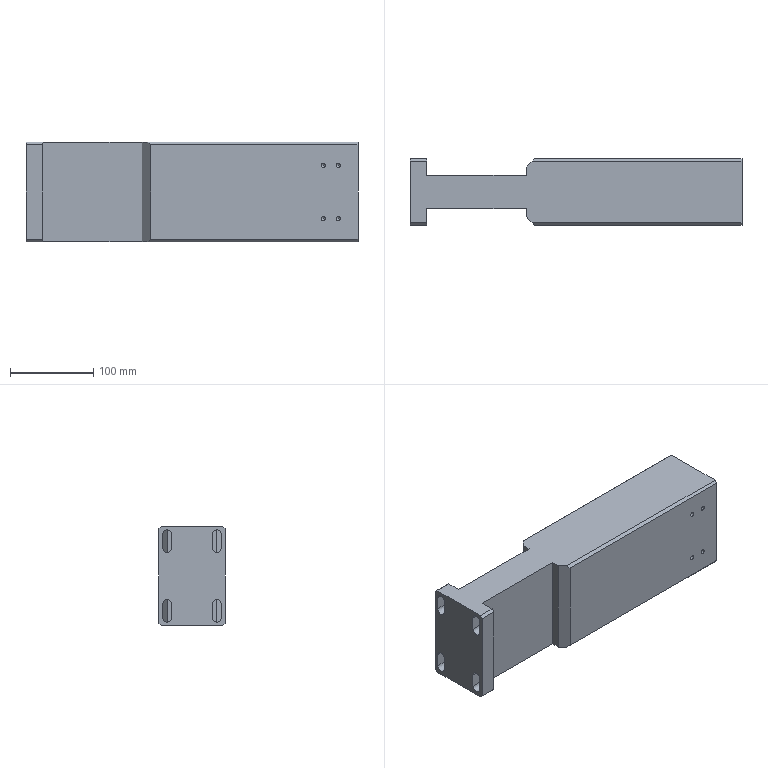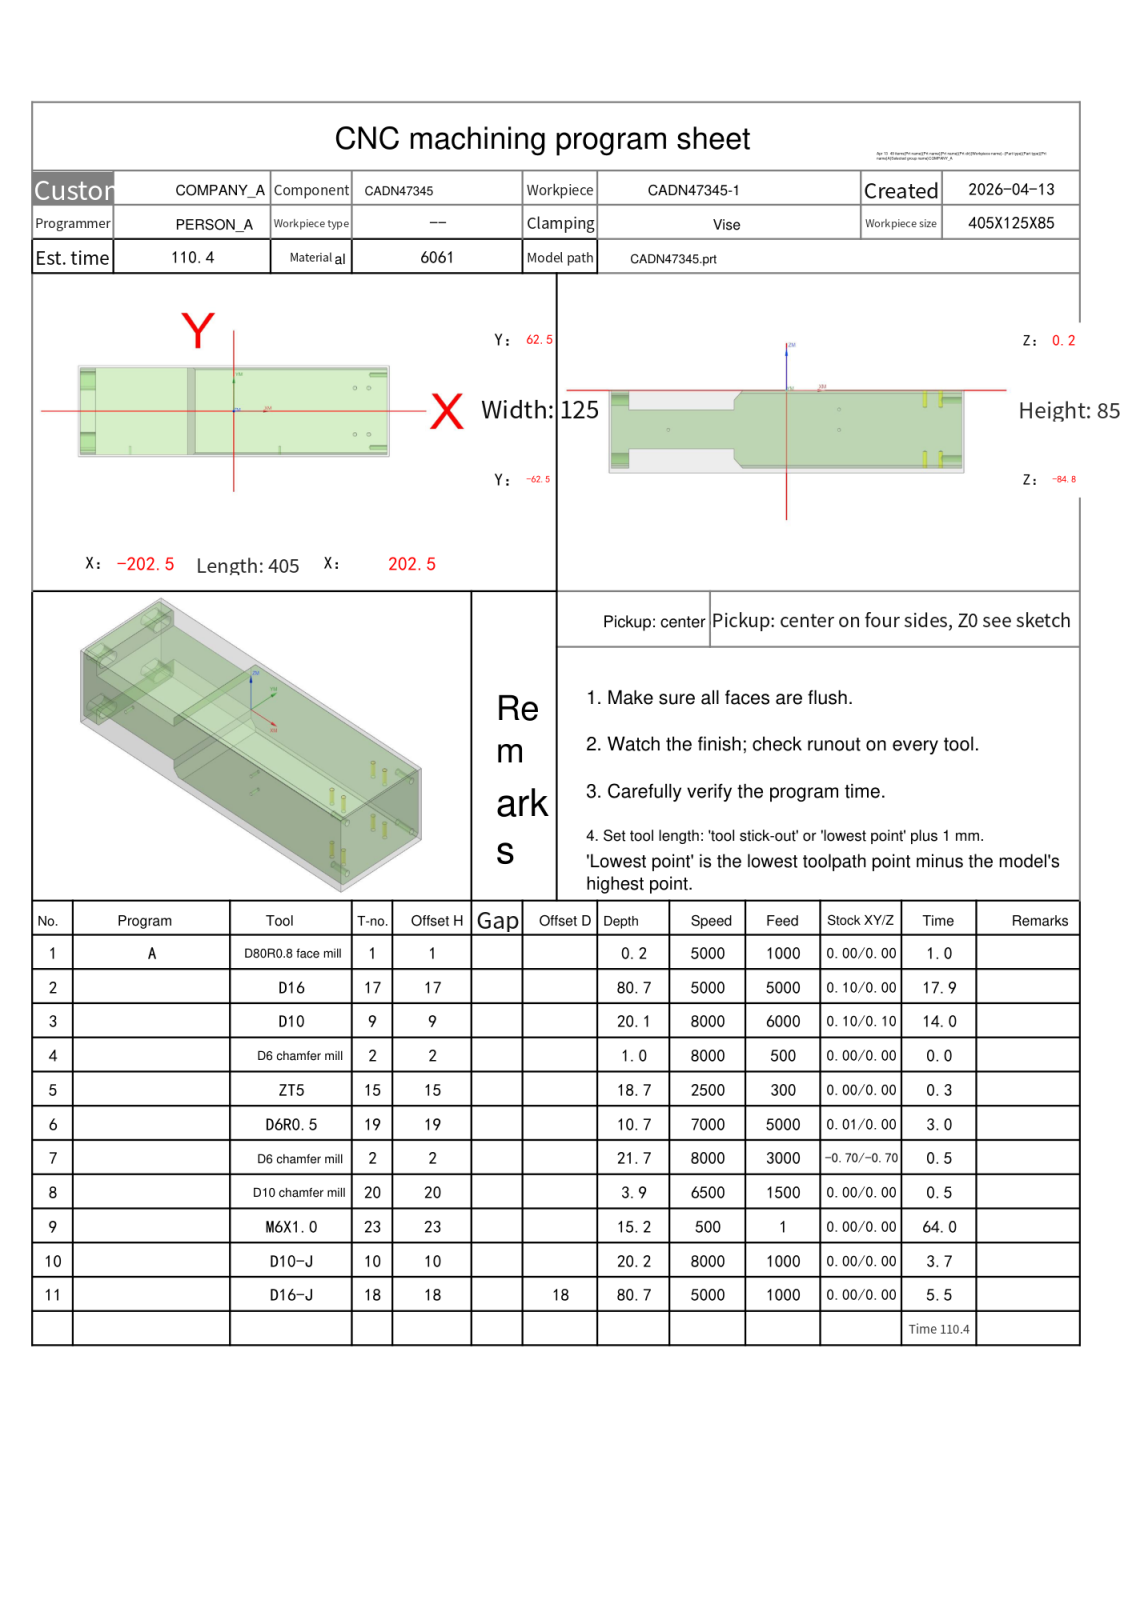NC program | NX | posted by the shop | part box 400 x 80 x 120 mm
Lines 711 to 1813 of 5986:
N3 T09 M06
(D10  D=10. R=0. H=09 ce=0.10 di=0.10)
G00 G90 G54 X-108.313 Y-74.5 M03 S8000
G43 H09 Z10.2
M08
Z.615
G01 Z-.585 F6000.
Y-67.08
G03 X-115.313 Y-60.08 I-7. J0.0
G01 X-174.823
G02 X-175.832 Y-63. I-5.247 J.18
G01 X-176.386
G02 X-180. Y-64.127 I-3.678 J5.437
G01 X-199.92
Y-63.
X-200.08
Y-62.727
X-199.921
X-199.92 Y-62.728
X-180. Y-62.727
G03 X-174.9 Y-57.585 I-.064 J5.164
G01 Y57.585
G03 X-180. Y62.727 I-5.164 J-.022
G01 X-199.92
X-199.921
X-199.999
X-200. Y62.728
X-200.001 Y62.727
X-200.08
Y63.
X-200.
Y64.127
Y63.
X-199.92
Y64.127
X-179.983
G02 X-176.386 Y63. I-.082 J-6.564
G01 X-175.849
G02 X-174.823 Y60.08 I-4.506 J-3.224
G01 X-174.002
X-166.904
X-65.09 Y60.082
X-64.793 Y60.08
X-58.152
G02 X-57.118 Y63. I5.554 J-.323
G01 X-54.305
G02 X-50.656 Y64.127 I3.649 J-5.344
G01 X200.011
X200.002 Y63.
X200.08
Y62.727
X200.001
X200. Y62.728
X-50.656 Y62.727
G03 X-55.727 Y57.656 I0.0 J-5.071
G01 Y-57.656
G03 X-50.656 Y-62.727 I5.071 J0.0
G01 X199.92
X199.921
X200.08
Y-63.
X199.92
Y-64.127
X-50.656
G02 X-54.305 Y-63. I0.0 J6.471
G01 X-57.118
G02 X-58.152 Y-60.08 I4.517 J3.243
G01 X-64.793
X-65.139 Y-60.082
X-65.389 Y-60.08
X-112.299
G02 X-113.112 Y-59.662 I.001 J1.
G01 X-117.515 Y-53.498
G03 X-118.327 Y-53.08 I-.813 J-.582
G01 X-166.904
G02 X-167.9 Y-52.084 I.004 J1.
G01 Y52.084
G02 X-166.904 Y53.08 I1. J-.004
G01 X-65.135 Y53.082
X-64.817 Y53.08
X-63.723
G02 X-62.727 Y52.084 I-.004 J-1.
G01 Y-52.084
G02 X-63.723 Y-53.08 I-1. J.004
G01 X-64.817
X-65.092 Y-53.082
X-65.366 Y-53.08
X-112.299
G02 X-113.112 Y-52.662 I.001 J1.
G01 X-117.515 Y-46.498
G03 X-118.327 Y-46.08 I-.813 J-.582
G01 X-159.905
G02 X-160.9 Y-45.085 I.005 J1.
G01 Y45.085
G02 X-159.905 Y46.08 I1. J-.005
G01 X-70.722 Y46.082
G02 X-69.727 Y45.087 I-.005 J-1.
G01 Y-45.085
G02 X-70.722 Y-46.08 I-1. J.005
G01 X-112.299
G02 X-113.112 Y-45.662 I.001 J1.
G01 X-117.515 Y-39.498
G03 X-118.327 Y-39.08 I-.813 J-.582
G01 X-152.905
G02 X-153.9 Y-38.085 I.005 J1.
G01 Y38.085
G02 X-152.905 Y39.08 I1. J-.005
G01 X-77.722 Y39.082
G02 X-76.727 Y38.087 I-.005 J-1.
G01 Y-38.085
G02 X-77.722 Y-39.08 I-1. J.005
G01 X-112.299
G02 X-113.112 Y-38.662 I0.0 J1.
G01 X-117.514 Y-32.498
G03 X-118.328 Y-32.08 I-.813 J-.582
G01 X-145.905
G02 X-146.9 Y-31.085 I.005 J1.
G01 Y31.086
G02 X-145.905 Y32.081 I1. J-.005
G01 X-84.722 Y32.082
G02 X-83.727 Y31.087 I-.005 J-1.
G01 Y-31.085
G02 X-84.722 Y-32.08 I-1. J.005
G01 X-112.299
G02 X-113.112 Y-31.662 I0.0 J1.
G01 X-117.514 Y-25.498
G03 X-118.328 Y-25.08 I-.814 J-.582
G01 X-138.905
G02 X-139.9 Y-24.085 I.005 J1.
G01 Y24.086
G02 X-138.905 Y25.081 I1. J-.005
G01 X-91.722 Y25.082
G02 X-90.727 Y24.087 I-.005 J-1.
G01 Y-24.085
G02 X-91.722 Y-25.08 I-1. J.005
G01 X-112.299
G02 X-113.112 Y-24.662 I0.0 J1.
G01 X-117.514 Y-18.498
G03 X-118.328 Y-18.08 I-.814 J-.582
G01 X-131.905
G02 X-132.9 Y-17.085 I.005 J1.
G01 Y17.086
G02 X-131.905 Y18.081 I1. J-.005
G01 X-98.721
G02 X-97.727 Y17.087 I-.005 J-1.
G01 Y-17.085
G02 X-98.721 Y-18.08 I-1. J.005
G01 X-112.299
G02 X-113.112 Y-17.662 I0.0 J1.
G01 X-117.514 Y-11.499
G03 X-118.328 Y-11.08 I-.814 J-.581
G01 X-124.905
G02 X-125.9 Y-10.085 I.005 J1.
G01 Y10.086
G02 X-124.905 Y11.081 I1. J-.005
G01 X-105.721
G02 X-104.727 Y10.087 I-.005 J-1.
G01 Y-10.085
G02 X-105.721 Y-11.08 I-1. J.005
G01 X-112.299
G02 X-113.112 Y-10.662 I0.0 J1.
G01 X-117.554 Y-4.443
G03 X-118.134 Y-4.052 I-.814 J-.582
G02 X-118.9 Y-3.085 I.234 J.972
G01 Y3.087
G02 X-117.905 Y4.081 I1. J-.005
G01 X-112.721
G02 X-111.727 Y3.087 I-.005 J-1.
G01 Y-3.085
G02 X-112.721 Y-4.08 I-1. J.005
G01 X-115.313
X-115.813
G03 X-122.813 Y-11.08 I0.0 J-7.
G01 Z.615
G00 Z3.
G01 X-108.313 Y-74.5
G00 Z.029
G01 Z-1.171
Y-67.08
G03 X-115.313 Y-60.08 I-7. J0.0
G01 X-174.823
G02 X-176.217 Y-63.466 I-5.247 J.18
X-180. Y-64.712 I-3.848 J5.318
G01 X-200.025
X-200. Y-63.312
X-180.
G03 X-174.9 Y-58.171 I-.064 J5.164
G01 Y58.171
G03 X-180. Y63.312 I-5.164 J-.022
G01 X-199.92
Y64.712
X-179.983
G02 X-176.234 Y63.479 I-.082 J-6.564
X-174.823 Y60.08 I-4.121 J-3.703
G01 X-166.905
X-65.09 Y60.082
X-64.793 Y60.08
X-58.152
G02 X-57.118 Y63. I5.554 J-.323
G01 X-55.626
G02 X-51.241 Y64.712 I4.385 J-4.759
G01 X199.92
Y63.312
X-51.241
G03 X-56.312 Y58.241 I0.0 J-5.071
G01 Y-58.241
G03 X-51.241 Y-63.312 I5.071 J0.0
G01 X200.
Y-64.712
X-51.241
G02 X-55.626 Y-63. I0.0 J6.471
G01 X-57.118
G02 X-58.152 Y-60.08 I4.517 J3.243
G01 X-64.793
X-65.139 Y-60.082
X-65.389 Y-60.08
X-112.299
G02 X-113.112 Y-59.662 I.001 J1.
G01 X-117.514 Y-53.499
G03 X-118.327 Y-53.081 I-.813 J-.582
G01 X-166.905 Y-53.08
G02 X-167.9 Y-52.085 I.005 J1.
G01 Y52.085
G02 X-166.905 Y53.08 I1. J-.005
G01 X-65.135 Y53.082
X-64.817 Y53.08
X-64.307
G02 X-63.312 Y52.084 I-.005 J-1.
G01 Y-52.084
G02 X-64.307 Y-53.08 I-1. J.005
G01 X-64.817
X-65.092 Y-53.082
X-112.299 Y-53.081
G02 X-113.112 Y-52.663 I.001 J1.
G01 X-117.514 Y-46.499
G03 X-118.327 Y-46.081 I-.813 J-.582
G01 X-159.905 Y-46.08
G02 X-160.9 Y-45.085 I.005 J1.
G01 Y45.085
G02 X-159.905 Y46.08 I1. J-.005
G01 X-71.307 Y46.082
G02 X-70.312 Y45.087 I-.005 J-1.
G01 Y-45.087
G02 X-71.307 Y-46.082 I-1. J.005
G01 X-112.299 Y-46.081
G02 X-113.112 Y-45.663 I.001 J1.
G01 X-117.514 Y-39.499
G03 X-118.327 Y-39.081 I-.813 J-.582
G01 X-152.905 Y-39.08
G02 X-153.9 Y-38.085 I.005 J1.
G01 Y38.086
G02 X-152.905 Y39.08 I1. J-.005
G01 X-78.307 Y39.082
G02 X-77.312 Y38.087 I-.005 J-1.
G01 Y-38.087
G02 X-78.307 Y-39.082 I-1. J.005
G01 X-112.299 Y-39.081
G02 X-113.112 Y-38.663 I.001 J1.
G01 X-117.514 Y-32.499
G03 X-118.327 Y-32.081 I-.813 J-.582
G01 X-145.905 Y-32.08
G02 X-146.9 Y-31.086 I.005 J1.
G01 Y31.086
G02 X-145.905 Y32.081 I1. J-.005
G01 X-85.307 Y32.082
G02 X-84.312 Y31.087 I-.005 J-1.
G01 Y-31.087
G02 X-85.307 Y-32.081 I-1. J.005
G01 X-112.299
G02 X-113.112 Y-31.663 I0.0 J1.
G01 X-117.514 Y-25.499
G03 X-118.327 Y-25.081 I-.814 J-.582
G01 X-138.906
G02 X-139.9 Y-24.086 I.006 J1.
G01 Y24.086
G02 X-138.906 Y25.081 I1. J-.005
G01 X-92.307 Y25.082
G02 X-91.312 Y24.087 I-.005 J-1.
G01 Y-24.087
G02 X-92.307 Y-25.081 I-1. J.005
G01 X-112.299
G02 X-113.112 Y-24.663 I0.0 J1.
G01 X-117.514 Y-18.499
G03 X-118.327 Y-18.081 I-.814 J-.582
G01 X-131.906
G02 X-132.9 Y-17.086 I.006 J1.
G01 Y17.086
G02 X-131.906 Y18.081 I1. J-.006
G01 X-99.306
G02 X-98.312 Y17.087 I-.006 J-1.
G01 Y-17.087
G02 X-99.306 Y-18.081 I-1. J.006
G01 X-112.298
G02 X-113.111 Y-17.663 I0.0 J1.
G01 X-117.514 Y-11.499
G03 X-118.327 Y-11.081 I-.814 J-.581
G01 X-124.906
G02 X-125.9 Y-10.086 I.006 J1.
G01 Y10.087
G02 X-124.906 Y11.081 I1. J-.006
G01 X-106.306
G02 X-105.312 Y10.087 I-.006 J-1.
G01 Y-10.087
G02 X-106.306 Y-11.081 I-1. J.006
G01 X-112.298
G02 X-113.111 Y-10.662 I0.0 J1.
G01 X-117.553 Y-4.444
G03 X-118.133 Y-4.053 I-.814 J-.581
G02 X-118.9 Y-3.087 I.233 J.972
G01 Y3.087
G02 X-117.906 Y4.081 I1. J-.006
G01 X-113.306
G02 X-112.312 Y3.087 I-.006 J-1.
G01 Y-3.087
G02 X-113.306 Y-4.081 I-1. J.006
G01 X-115.312
X-115.812
G03 X-122.812 Y-11.081 I0.0 J-7.
G01 Z.029
G00 Z3.
G01 X-108.313 Y-74.5
G00 Z-.556
G01 Z-1.756
Y-67.08
G03 X-115.313 Y-60.08 I-7. J0.0
G01 X-174.823
G02 X-180.07 Y-65.151 I-5.247 J.18
G01 X-180.08
X-200.
X-200.085 Y-65.156
X-200.08 Y-65.071
Y-63.897
X-199.92
X-180.
G03 X-174.9 Y-58.756 I-.064 J5.164
G01 Y58.756
G03 X-180. Y63.897 I-5.164 J-.022
G01 X-199.92
X-200.
X-200.08
Y65.071
X-200.085 Y65.156
X-200. Y65.151
X-180.079
G02 X-177.129 Y64.28 I-.06 J-5.639
X-174.823 Y60.08 I-3.226 J-4.504
G01 X-166.904
X-65.09 Y60.082
X-64.793 Y60.08
X-58.152
G02 X-55.897 Y64.236 I5.554 J-.324
X-52.574 Y65.157 I3.324 J-5.531
X-52.279 Y65.151 I0.0 J-6.453
G01 X200.
X200.085 Y65.156
X200.08 Y65.071
Y63.897
X199.92
X-51.827
G03 X-56.897 Y58.827 I0.0 J-5.071
G01 Y-58.827
G03 X-51.827 Y-63.897 I5.071 J0.0
G01 X200.
X200.08
Y-64.215
Y-65.071
X200.085 Y-65.156
X200. Y-65.151
X-52.283
X-53.186 Y-65.128
X-54.093 Y-64.999
X-54.999 Y-64.705
X-55.835 Y-64.281
G02 X-58.152 Y-60.08 I3.234 J4.523
G01 X-64.837
X-65.139 Y-60.082
X-65.389 Y-60.08
X-112.299
G02 X-113.112 Y-59.662 I.001 J1.
G01 X-117.515 Y-53.498
G03 X-118.327 Y-53.08 I-.813 J-.582
G01 X-166.904
G02 X-167.9 Y-52.084 I.004 J1.
G01 Y52.084
G02 X-166.904 Y53.08 I1. J-.004
G01 X-65.135 Y53.082
X-64.886 Y53.08
G02 X-63.897 Y52.084 I-.011 J-1.
G01 Y-52.084
G02 X-64.886 Y-53.08 I-1. J.004
G01 X-65.092 Y-53.082
X-65.366 Y-53.08
X-112.299
G02 X-113.112 Y-52.662 I.001 J1.
G01 X-117.515 Y-46.498
G03 X-118.327 Y-46.08 I-.813 J-.582
G01 X-159.905
G02 X-160.9 Y-45.085 I.005 J1.
G01 Y45.085
G02 X-159.905 Y46.08 I1. J-.005
G01 X-71.893 Y46.082
G02 X-70.897 Y45.087 I-.004 J-1.
G01 Y-45.085
G02 X-71.893 Y-46.08 I-1. J.005
G01 X-112.299
G02 X-113.112 Y-45.662 I0.0 J1.
G01 X-117.514 Y-39.498
G03 X-118.327 Y-39.08 I-.813 J-.582
G01 X-152.905
G02 X-153.9 Y-38.085 I.005 J1.
G01 Y38.085
G02 X-152.905 Y39.08 I1. J-.005
G01 X-78.893 Y39.082
G02 X-77.897 Y38.087 I-.005 J-1.
G01 Y-38.085
G02 X-78.893 Y-39.08 I-1. J.005
G01 X-112.299
G02 X-113.112 Y-38.662 I0.0 J1.
G01 X-117.514 Y-32.498
G03 X-118.328 Y-32.08 I-.813 J-.582
G01 X-145.905
G02 X-146.9 Y-31.085 I.005 J1.
G01 Y31.085
G02 X-145.905 Y32.081 I1. J-.005
G01 X-85.892 Y32.082
G02 X-84.897 Y31.087 I-.005 J-1.
G01 Y-31.085
G02 X-85.892 Y-32.08 I-1. J.005
G01 X-112.299
G02 X-113.112 Y-31.662 I0.0 J1.
G01 X-117.514 Y-25.498
G03 X-118.328 Y-25.08 I-.814 J-.582
G01 X-138.905
G02 X-139.9 Y-24.085 I.005 J1.
G01 Y24.086
G02 X-138.905 Y25.081 I1. J-.005
G01 X-92.892 Y25.082
G02 X-91.897 Y24.087 I-.005 J-1.
G01 Y-24.085
G02 X-92.892 Y-25.08 I-1. J.005
G01 X-112.299
G02 X-113.112 Y-24.662 I0.0 J1.
G01 X-117.514 Y-18.498
G03 X-118.328 Y-18.08 I-.814 J-.582
G01 X-131.905
G02 X-132.9 Y-17.085 I.005 J1.
G01 Y17.086
G02 X-131.905 Y18.081 I1. J-.005
G01 X-99.892
G02 X-98.897 Y17.087 I-.005 J-1.
G01 Y-17.085
G02 X-99.892 Y-18.08 I-1. J.005
G01 X-112.299
G02 X-113.112 Y-17.662 I0.0 J1.
G01 X-117.514 Y-11.499
G03 X-118.328 Y-11.08 I-.814 J-.582
G01 X-124.905
G02 X-125.9 Y-10.085 I.005 J1.
G01 Y10.086
G02 X-124.905 Y11.081 I1. J-.005
G01 X-106.892
G02 X-105.897 Y10.087 I-.005 J-1.
G01 Y-10.085
G02 X-106.892 Y-11.08 I-1. J.005
G01 X-112.299
G02 X-113.112 Y-10.661 I0.0 J1.
G01 X-117.554 Y-4.443
G03 X-118.134 Y-4.052 I-.814 J-.582
G02 X-118.9 Y-3.085 I.234 J.972
G01 Y3.086
G02 X-117.905 Y4.081 I1. J-.005
G01 X-113.892
G02 X-112.897 Y3.087 I-.005 J-1.
G01 Y-3.085
G02 X-113.892 Y-4.08 I-1. J.005
G01 X-115.313
X-115.813
G03 X-122.813 Y-11.08 I0.0 J-7.
G01 Z-.556
G00 Z3.
G01 X-108.313 Y-74.5
G00 Z-1.141
G01 Z-2.341
Y-67.08
G03 X-115.313 Y-60.08 I-7. J0.0
G01 X-174.823
G02 X-180.07 Y-65.151 I-5.247 J.18
G01 X-180.08
X-200.
X-200.085 Y-65.156
X-200.08 Y-65.071
Y-64.483
X-200.
X-199.92
X-180.
G03 X-174.9 Y-59.341 I-.069 J5.168
G01 Y59.341
G03 X-180. Y64.483 I-5.168 J-.027
G01 X-199.92
X-200.
X-200.08
Y65.071
X-200.085 Y65.156
X-200. Y65.151
X-180.079
G02 X-177.129 Y64.28 I-.06 J-5.639
X-174.823 Y60.08 I-3.226 J-4.504
G01 X-65.09 Y60.082
X-64.793 Y60.08
X-58.152
G02 X-55.897 Y64.236 I5.554 J-.324
X-52.574 Y65.157 I3.324 J-5.531
X-52.279 Y65.151 I0.0 J-6.453
G01 X200.
X200.085 Y65.156
X200.08 Y65.071
Y64.483
X200.
X-52.412
G03 X-57.483 Y59.412 I0.0 J-5.071
G01 Y-59.412
G03 X-52.412 Y-64.483 I5.071 J0.0
G01 X199.92
X200.
X200.08
Y-65.071
X200.085 Y-65.156
X200. Y-65.151
X-52.283
X-53.186 Y-65.128
X-54.093 Y-64.999
X-54.999 Y-64.705
X-55.835 Y-64.281
G02 X-58.152 Y-60.08 I3.234 J4.523
G01 X-64.793
X-65.092 Y-60.082
X-65.478 Y-60.08
X-112.299
G02 X-113.112 Y-59.662 I.001 J1.
G01 X-117.515 Y-53.498
G03 X-118.327 Y-53.08 I-.813 J-.582
G01 X-166.904
G02 X-167.9 Y-52.084 I.004 J1.
G01 Y52.085
G02 X-166.904 Y53.08 I1. J-.004
G01 X-65.478 Y53.082
G02 X-64.483 Y52.087 I-.004 J-1.
G01 Y-52.084
G02 X-65.478 Y-53.08 I-1. J.004
G01 X-112.299
G02 X-113.112 Y-52.662 I.001 J1.
G01 X-117.515 Y-46.498
G03 X-118.328 Y-46.08 I-.813 J-.582
G01 X-159.905
G02 X-160.9 Y-45.085 I.005 J1.
G01 Y45.085
G02 X-159.905 Y46.08 I1. J-.005
G01 X-72.478 Y46.082
G02 X-71.483 Y45.087 I-.005 J-1.
G01 Y-45.085
G02 X-72.478 Y-46.08 I-1. J.005
G01 X-112.299
G02 X-113.112 Y-45.662 I.001 J1.
G01 X-117.515 Y-39.498
G03 X-118.327 Y-39.08 I-.813 J-.582
G01 X-152.905
G02 X-153.9 Y-38.085 I.005 J1.
G01 Y38.086
G02 X-152.905 Y39.08 I1. J-.005
G01 X-79.477 Y39.082
G02 X-78.483 Y38.087 I-.005 J-1.
G01 Y-38.085
G02 X-79.477 Y-39.08 I-1. J.005
G01 X-112.299
G02 X-113.112 Y-38.662 I0.0 J1.
G01 X-117.515 Y-32.498
G03 X-118.328 Y-32.08 I-.813 J-.582
G01 X-145.905
G02 X-146.9 Y-31.085 I.005 J1.
G01 Y31.086
G02 X-145.905 Y32.081 I1. J-.005
G01 X-86.477 Y32.082
G02 X-85.483 Y31.087 I-.005 J-1.
G01 Y-31.085
G02 X-86.477 Y-32.08 I-1. J.005
G01 X-112.299
G02 X-113.112 Y-31.662 I0.0 J1.
G01 X-117.514 Y-25.498
G03 X-118.328 Y-25.08 I-.814 J-.582
G01 X-138.905
G02 X-139.9 Y-24.085 I.005 J1.
G01 Y24.086
G02 X-138.905 Y25.081 I1. J-.005
G01 X-93.477 Y25.082
G02 X-92.483 Y24.087 I-.005 J-1.
G01 Y-24.085
G02 X-93.477 Y-25.08 I-1. J.005
G01 X-112.299
G02 X-113.112 Y-24.662 I0.0 J1.
G01 X-117.514 Y-18.498
G03 X-118.328 Y-18.08 I-.814 J-.582
G01 X-131.906
G02 X-132.9 Y-17.086 I.006 J1.
G01 Y17.086
G02 X-131.906 Y18.081 I1. J-.006
G01 X-100.477
G02 X-99.483 Y17.087 I-.006 J-1.
G01 Y-17.086
G02 X-100.477 Y-18.08 I-1. J.006
G01 X-112.299
G02 X-113.112 Y-17.662 I0.0 J1.
G01 X-117.514 Y-11.499
G03 X-118.328 Y-11.08 I-.814 J-.582
G01 X-124.906
G02 X-125.9 Y-10.086 I.006 J1.
G01 Y10.087
G02 X-124.906 Y11.081 I1. J-.006
G01 X-107.477
G02 X-106.483 Y10.087 I-.006 J-1.
G01 Y-10.086
G02 X-107.477 Y-11.08 I-1. J.006
G01 X-112.299
G02 X-113.112 Y-10.661 I0.0 J1.
G01 X-117.554 Y-4.443
G03 X-118.134 Y-4.052 I-.814 J-.582
G02 X-118.9 Y-3.086 I.234 J.972
G01 Y3.087
G02 X-117.906 Y4.081 I1. J-.006
G01 X-114.477
G02 X-113.483 Y3.087 I-.006 J-1.
G01 Y-3.086
G02 X-114.477 Y-4.08 I-1. J.006
G01 X-115.313
X-115.813
G03 X-122.813 Y-11.08 I0.0 J-7.
G01 Z-1.141
G00 Z3.
G01 X-108.313 Y-74.5
G00 Z-1.726
G01 Z-2.926
Y-67.08
G03 X-115.313 Y-60.08 I-7. J0.0
G01 X-174.823
G02 X-175.832 Y-63. I-5.247 J.18
X-180.07 Y-65.151 I-4.238 J3.1
G01 X-180.08
X-200.
X-200.076 Y-65.163
X-200.078 Y-65.086
Y-65.067
X-180. Y-65.068
G03 X-174.9 Y-59.947 I-.021 J5.121
G01 Y-59.927
Y59.927
Y59.947
G03 X-180. Y65.068 I-5.121 J0.0
G01 X-200.078 Y65.067
X-200.079 Y65.086
X-200.076 Y65.163
X-200. Y65.151
X-180.079
G02 X-177.129 Y64.28 I-.06 J-5.639
X-175.849 Y63. I-3.226 J-4.504
X-174.823 Y60.08 I-4.506 J-3.224
G01 X-166.906
X-65.068 Y60.082
X-64.793 Y60.08
X-58.152
X-58.141 Y60.228
X-58.054 Y60.221
X-58.068 Y59.997
Y-59.997
X-58.053 Y-60.22
X-58.141 Y-60.226
X-58.152 Y-60.08
X-64.793
X-65.092 Y-60.082
X-65.389 Y-60.08
X-112.299
G02 X-113.112 Y-59.662 I.001 J1.
G01 X-117.515 Y-53.498
G03 X-118.327 Y-53.08 I-.813 J-.582
G01 X-166.905
G02 X-167.9 Y-52.085 I.005 J1.
G01 Y52.086
G02 X-166.905 Y53.08 I1. J-.005
G01 X-66.063 Y53.082
G02 X-65.068 Y52.087 I-.005 J-1.
G01 Y-52.085
G02 X-66.063 Y-53.08 I-1. J.005
G01 X-112.299
G02 X-113.112 Y-52.662 I.001 J1.
G01 X-117.515 Y-46.498
G03 X-118.327 Y-46.08 I-.813 J-.582
G01 X-159.906
G02 X-160.9 Y-45.086 I.006 J1.
G01 Y45.086
G02 X-159.906 Y46.08 I1. J-.006
G01 X-73.062 Y46.082
G02 X-72.068 Y45.088 I-.006 J-1.
G01 Y-45.086
G02 X-73.062 Y-46.08 I-1. J.006
G01 X-112.299
G02 X-113.112 Y-45.662 I.001 J1.
G01 X-117.515 Y-39.498
G03 X-118.327 Y-39.08 I-.813 J-.582
G01 X-152.906
G02 X-153.9 Y-38.086 I.006 J1.
G01 Y38.086
G02 X-152.906 Y39.08 I1. J-.006
G01 X-80.062 Y39.082
G02 X-79.068 Y38.088 I-.006 J-1.
G01 Y-38.086
G02 X-80.062 Y-39.08 I-1. J.006
G01 X-112.299
G02 X-113.112 Y-38.662 I0.0 J1.
G01 X-117.514 Y-32.498
G03 X-118.328 Y-32.08 I-.813 J-.582
G01 X-145.906
G02 X-146.9 Y-31.086 I.006 J1.
G01 Y31.086
G02 X-145.906 Y32.081 I1. J-.006
G01 X-87.062 Y32.082
G02 X-86.068 Y31.088 I-.006 J-1.
G01 Y-31.086
G02 X-87.062 Y-32.08 I-1. J.006
G01 X-112.299
G02 X-113.112 Y-31.662 I0.0 J1.
G01 X-117.514 Y-25.498
G03 X-118.328 Y-25.08 I-.814 J-.582
G01 X-138.906
G02 X-139.9 Y-24.086 I.006 J1.
G01 Y24.087
G02 X-138.906 Y25.081 I1. J-.006
G01 X-94.062 Y25.082
G02 X-93.068 Y24.088 I-.006 J-1.
G01 Y-24.086
G02 X-94.062 Y-25.08 I-1. J.006
G01 X-112.299
G02 X-113.112 Y-24.662 I0.0 J1.
G01 X-117.514 Y-18.498
G03 X-118.328 Y-18.08 I-.814 J-.582
G01 X-131.906
G02 X-132.9 Y-17.086 I.006 J1.
G01 Y17.087
G02 X-131.906 Y18.081 I1. J-.006
G01 X-101.062
G02 X-100.068 Y17.088 I-.006 J-1.
G01 Y-17.086
G02 X-101.062 Y-18.08 I-1. J.006
G01 X-112.299
G02 X-113.112 Y-17.662 I0.0 J1.
G01 X-117.514 Y-11.499
G03 X-118.328 Y-11.08 I-.814 J-.581
G01 X-124.906
G02 X-125.9 Y-10.086 I.006 J1.
G01 Y10.087
G02 X-124.906 Y11.081 I1. J-.006
G01 X-108.062
G02 X-107.068 Y10.087 I-.006 J-1.
G01 Y-10.086
G02 X-108.062 Y-11.08 I-1. J.006
G01 X-112.299
G02 X-113.112 Y-10.661 I0.0 J1.
G01 X-117.554 Y-4.443
G03 X-118.134 Y-4.052 I-.814 J-.582
G02 X-118.9 Y-3.086 I.234 J.972
G01 Y3.087
G02 X-117.906 Y4.081 I1. J-.006
G01 X-115.062
G02 X-114.068 Y3.087 I-.006 J-1.
G01 Y-3.086
G02 X-115.062 Y-4.08 I-1. J.006
G01 X-115.313
X-115.813
G03 X-122.813 Y-11.08 I0.0 J-7.
G01 Z-1.726
G00 Z3.
G01 X-108.313 Y-74.5
G00 Z-2.312
G01 Z-3.512
Y-67.08
G03 X-115.313 Y-60.08 I-7. J0.0
G01 X-174.823
X-174.9 Y-60.058
Y-59.927
Y60.068
X-174.823 Y60.08
X-65.09 Y60.082
X-64.793 Y60.08
X-58.653
Y59.92
Y-59.92
Y-60.08
X-64.793
X-65.092 Y-60.082
X-65.389 Y-60.08
X-112.299
G02 X-113.112 Y-59.662 I.001 J1.
G01 X-117.515 Y-53.498
G03 X-118.327 Y-53.08 I-.813 J-.582
G01 X-166.905
G02 X-167.9 Y-52.085 I.005 J1.
G01 Y52.085
G02 X-166.905 Y53.08 I1. J-.005
G01 X-66.648 Y53.082
G02 X-65.653 Y52.087 I-.005 J-1.
G01 Y-52.085
G02 X-66.648 Y-53.08 I-1. J.005
G01 X-112.299
G02 X-113.112 Y-52.662 I.001 J1.
G01 X-117.515 Y-46.498
G03 X-118.327 Y-46.08 I-.813 J-.582
G01 X-159.905
G02 X-160.9 Y-45.085 I.005 J1.
G01 Y45.086
G02 X-159.905 Y46.08 I1. J-.005
G01 X-73.648 Y46.082
G02 X-72.653 Y45.087 I-.005 J-1.
G01 Y-45.085
G02 X-73.648 Y-46.08 I-1. J.005
G01 X-112.299
G02 X-113.112 Y-45.662 I.001 J1.
G01 X-117.515 Y-39.498
G03 X-118.327 Y-39.08 I-.813 J-.582
G01 X-152.906
G02 X-153.9 Y-38.086 I.006 J1.
G01 Y38.086
G02 X-152.906 Y39.08 I1. J-.006
G01 X-80.648 Y39.082
G02 X-79.653 Y38.087 I-.006 J-1.
G01 Y-38.086
G02 X-80.648 Y-39.08 I-1. J.006
G01 X-112.299
G02 X-113.112 Y-38.662 I0.0 J1.
G01 X-117.514 Y-32.498
G03 X-118.328 Y-32.08 I-.813 J-.582
G01 X-145.906
G02 X-146.9 Y-31.086 I.006 J1.
G01 Y31.086
G02 X-145.906 Y32.081 I1. J-.006
G01 X-87.647 Y32.082
G02 X-86.653 Y31.087 I-.006 J-1.
G01 Y-31.086
G02 X-87.647 Y-32.08 I-1. J.006
G01 X-112.299
G02 X-113.112 Y-31.662 I0.0 J1.
G01 X-117.514 Y-25.498
G03 X-118.328 Y-25.08 I-.814 J-.582
G01 X-138.906
G02 X-139.9 Y-24.086 I.006 J1.
G01 Y24.087
G02 X-138.906 Y25.081 I1. J-.006
G01 X-94.647 Y25.082
G02 X-93.653 Y24.087 I-.006 J-1.
G01 Y-24.086
G02 X-94.647 Y-25.08 I-1. J.006
G01 X-112.299
G02 X-113.112 Y-24.662 I0.0 J1.
G01 X-117.514 Y-18.498
G03 X-118.328 Y-18.08 I-.814 J-.582
G01 X-131.906
G02 X-132.9 Y-17.086 I.006 J1.
G01 Y17.087
G02 X-131.906 Y18.081 I1. J-.006
G01 X-101.647
G02 X-100.653 Y17.087 I-.006 J-1.
G01 Y-17.086
G02 X-101.647 Y-18.08 I-1. J.006
G01 X-112.299
G02 X-113.112 Y-17.662 I0.0 J1.
G01 X-117.514 Y-11.499
G03 X-118.328 Y-11.08 I-.814 J-.582
G01 X-124.906
G02 X-125.9 Y-10.086 I.006 J1.
G01 Y10.087
G02 X-124.906 Y11.081 I1. J-.006
G01 X-108.647
G02 X-107.653 Y10.087 I-.006 J-1.
G01 Y-10.086
G02 X-108.647 Y-11.08 I-1. J.006
G01 X-112.315
G02 X-113.113 Y-10.682 I0.0 J1.
G01 X-117.927 Y-4.299
G03 X-118.312 Y-3.991 I-.798 J-.602
G02 X-118.9 Y-3.086 I.412 J.911
G01 Y3.087
G02 X-117.906 Y4.081 I1. J-.006
G01 X-115.647
G02 X-114.653 Y3.087 I-.006 J-1.
G01 Y-3.086
G02 X-115.611 Y-4.079 I-1. J.006
G01 X-116.111 Y-4.08
G03 X-123.111 Y-11.08 I0.0 J-7.
G01 Z-2.312
G00 Z3.
G01 X-108.313 Y-74.5
G00 Z-2.897
G01 Z-4.097
Y-67.08
G03 X-115.313 Y-60.08 I-7. J0.0
G01 X-174.823
X-174.9 Y-60.057
Y-53.08
Y53.08
Y60.067
X-174.823 Y60.08
X-65.09 Y60.082
X-64.793 Y60.08
X-59.238
Y59.92
Y-59.92
Y-60.08
X-64.793
X-65.092 Y-60.082
X-65.389 Y-60.08
X-112.299
G02 X-113.112 Y-59.662 I.001 J1.
G01 X-117.515 Y-53.498
G03 X-118.327 Y-53.08 I-.813 J-.582
G01 X-166.906
G02 X-167.9 Y-52.086 I.006 J1.
G01 Y52.086
G02 X-166.906 Y53.08 I1. J-.006
G01 X-67.233 Y53.082
G02 X-66.238 Y52.088 I-.006 J-1.
G01 Y-52.086
G02 X-67.233 Y-53.08 I-1. J.006
G01 X-112.299
G02 X-113.112 Y-52.662 I.001 J1.
G01 X-117.515 Y-46.498
G03 X-118.327 Y-46.08 I-.813 J-.582
G01 X-159.906
G02 X-160.9 Y-45.086 I.006 J1.
G01 Y45.086
G02 X-159.906 Y46.08 I1. J-.006
G01 X-74.233 Y46.082
G02 X-73.238 Y45.088 I-.006 J-1.
G01 Y-45.086
G02 X-74.233 Y-46.08 I-1. J.006
G01 X-112.299
G02 X-113.112 Y-45.662 I.001 J1.
G01 X-117.514 Y-39.498
G03 X-118.327 Y-39.08 I-.813 J-.582
G01 X-152.906
G02 X-153.9 Y-38.086 I.006 J1.
G01 Y38.086
G02 X-152.906 Y39.08 I1. J-.006
G01 X-81.233 Y39.082
G02 X-80.238 Y38.088 I-.006 J-1.
G01 Y-38.086
G02 X-81.233 Y-39.08 I-1. J.006
G01 X-112.299
G02 X-113.112 Y-38.662 I0.0 J1.
G01 X-117.515 Y-32.498
G03 X-118.328 Y-32.08 I-.813 J-.582
G01 X-145.906
G02 X-146.9 Y-31.086 I.006 J1.
G01 Y31.087
G02 X-145.906 Y32.081 I1. J-.006
G01 X-88.232 Y32.082
G02 X-87.238 Y31.088 I-.006 J-1.
G01 Y-31.086
G02 X-88.232 Y-32.08 I-1. J.006
G01 X-112.299
G02 X-113.112 Y-31.662 I0.0 J1.
G01 X-117.514 Y-25.498
G03 X-118.328 Y-25.08 I-.814 J-.582
G01 X-138.906
G02 X-139.9 Y-24.086 I.006 J1.
G01 Y24.087
G02 X-138.906 Y25.081 I1. J-.006
G01 X-95.232 Y25.082
G02 X-94.238 Y24.088 I-.006 J-1.
G01 Y-24.086
G02 X-95.232 Y-25.08 I-1. J.006
G01 X-112.299
G02 X-113.112 Y-24.662 I0.0 J1.
G01 X-117.514 Y-18.498
G03 X-118.328 Y-18.08 I-.814 J-.582
G01 X-131.906
G02 X-132.9 Y-17.086 I.006 J1.
G01 Y17.087
G02 X-131.906 Y18.081 I1. J-.006
G01 X-102.232
G02 X-101.238 Y17.088 I-.006 J-1.
G01 Y-17.086
G02 X-102.232 Y-18.08 I-1. J.006
G01 X-112.299
G02 X-113.112 Y-17.662 I0.0 J1.
G01 X-117.514 Y-11.499
G03 X-118.328 Y-11.08 I-.814 J-.582
G01 X-124.906
G02 X-125.9 Y-10.086 I.006 J1.
G01 Y10.087
G02 X-124.906 Y11.081 I1. J-.006
G01 X-109.232
G02 X-108.238 Y10.088 I-.006 J-1.
G01 Y-10.086
G02 X-109.232 Y-11.08 I-1. J.006
G01 X-112.33
G02 X-113.113 Y-10.702 I0.0 J1.
G01 X-118.517 Y-3.887
X-118.6 Y-3.794
G02 X-118.9 Y-3.086 I.7 J.714
G01 Y3.088
G02 X-117.906 Y4.081 I1. J-.006
G01 X-116.232
G02 X-115.238 Y3.088 I-.006 J-1.
G01 Y-3.086
G02 X-116.124 Y-4.073 I-1. J.006
G01 X-116.232 Y-4.08
X-116.623
G03 X-123.623 Y-11.08 I0.0 J-7.
G01 Z-2.897
G00 Z3.
G01 X-108.313 Y-74.5
G00 Z-3.482
G01 Z-4.682
Y-67.08
G03 X-115.313 Y-60.08 I-7. J0.0
G01 X-174.823
X-174.9 Y-60.057
Y-53.08
Y53.08
Y60.066
X-174.823 Y60.08
X-65.09 Y60.082
X-64.793 Y60.08
X-59.824
Y59.92
Y-59.92
Y-60.08
X-64.793
X-65.092 Y-60.082
X-65.389 Y-60.08
X-112.299
G02 X-113.112 Y-59.662 I.001 J1.
G01 X-117.515 Y-53.498
G03 X-118.327 Y-53.08 I-.813 J-.582
G01 X-166.906
G02 X-167.9 Y-52.086 I.006 J1.
G01 Y52.086
G02 X-166.906 Y53.08 I1. J-.006
G01 X-67.818 Y53.082
G02 X-66.824 Y52.088 I-.006 J-1.
G01 Y-52.086
G02 X-67.818 Y-53.08 I-1. J.006
G01 X-112.299
G02 X-113.112 Y-52.662 I.001 J1.
G01 X-117.515 Y-46.498
G03 X-118.327 Y-46.08 I-.813 J-.582
G01 X-159.906
G02 X-160.9 Y-45.086 I.006 J1.
G01 Y45.086
G02 X-159.906 Y46.08 I1. J-.006
G01 X-74.818 Y46.082
G02 X-73.824 Y45.088 I-.006 J-1.
G01 Y-45.086
G02 X-74.818 Y-46.08 I-1. J.006
G01 X-112.299
G02 X-113.112 Y-45.662 I0.0 J1.
G01 X-117.515 Y-39.498
G03 X-118.327 Y-39.08 I-.813 J-.582
G01 X-152.906
G02 X-153.9 Y-38.086 I.006 J1.
G01 Y38.087
G02 X-152.906 Y39.08 I1. J-.006
G01 X-81.818 Y39.082
G02 X-80.824 Y38.088 I-.006 J-1.
G01 Y-38.086
G02 X-81.818 Y-39.08 I-1. J.006
G01 X-112.299
G02 X-113.112 Y-38.662 I.001 J1.
G01 X-117.514 Y-32.498
G03 X-118.328 Y-32.08 I-.813 J-.582
G01 X-145.906
G02 X-146.9 Y-31.086 I.006 J1.
G01 Y31.087
G02 X-145.906 Y32.081 I1. J-.006
G01 X-88.817 Y32.082
G02 X-87.824 Y31.088 I-.006 J-1.
G01 Y-31.086
G02 X-88.817 Y-32.08 I-1. J.006
G01 X-112.299
G02 X-113.112 Y-31.662 I0.0 J1.
G01 X-117.514 Y-25.498
G03 X-118.328 Y-25.08 I-.813 J-.582
G01 X-138.907
G02 X-139.9 Y-24.087 I.006 J1.
G01 Y24.087
G02 X-138.907 Y25.081 I1. J-.006
G01 X-95.817 Y25.082
G02 X-94.824 Y24.088 I-.006 J-1.
G01 Y-24.087
G02 X-95.817 Y-25.08 I-1. J.006
G01 X-112.299
G02 X-113.112 Y-24.662 I0.0 J1.
G01 X-117.514 Y-18.498
G03 X-118.328 Y-18.08 I-.814 J-.582
G01 X-131.907
G02 X-132.9 Y-17.087 I.007 J1.
G01 Y17.087